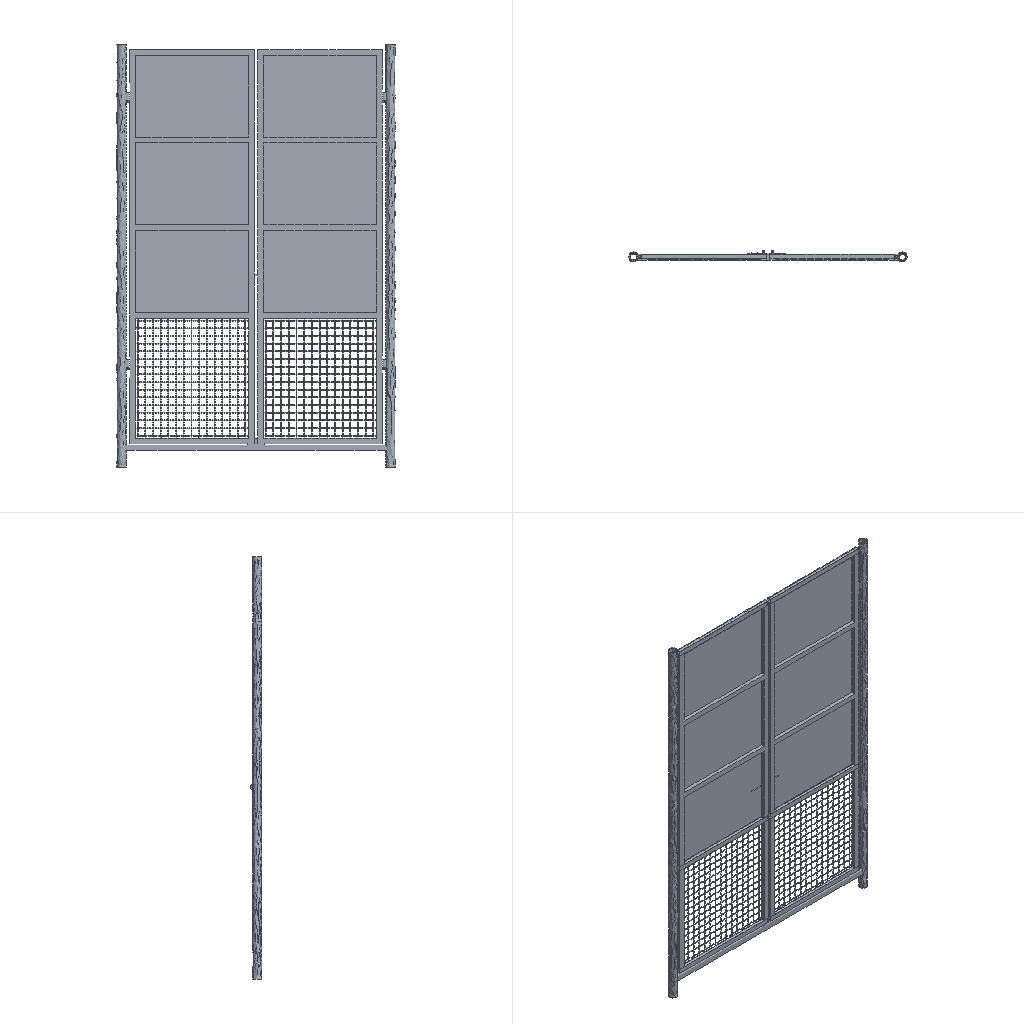Simulation study | ansys workbench
Ansys APDL input file, long lists of numbers shortened:
/batch
/config,noeldb,1     ! force off writing results to database
*get,_wallstrt,active,,time,wall
! ANSYS input file written by Workbench version 2022 R1
! File used for geometry attach:
/title,wbnew--____ (B5)
! ****** Begin Custom Load Command Snippet ******
/COM, ACT Extensions:
/COM,     LSDYNA, 2021.1
/COM,
! ****** End   Custom Load Command Snippet ******
*DIM,_wb_ProjectScratch_dir,string,248
_wb_ProjectScratch_dir(1) = ''
*DIM,_wb_SolverFiles_dir,string,248
_wb_SolverFiles_dir(1) = ''
*DIM,_wb_userfiles_dir,string,248
_wb_userfiles_dir(1) = ''
/com,--- Data in consistent NMM units. See Solving Units in the help system for more information.
/units,MPA
/nopr
/wb,file,start              !  signify a WB generated input file
/prep7
! Turn off shape checking because checks already performed inside WB mesher.
! See help system for more information.
SHPP,OFF,,NOWARN
/nolist
etcon,set             ! allow ANSYS to choose best KEYOP's for 180x elements, resets any applicable keyopt to MAPDL defaults
/com,*********** Nodes for the whole assembly ***********
nblock,3,,124940
(1i9,3e20.9e3)
    95183     1.797300000E+03     1.700000000E+01    -2.052050000E+03
! (113581 more lines like these left out)
-1
/wb,elem,start            !  set before creation of elements
/com,*********** Elements for Body 1 "SYS|__" ***********
et,1,187
eblock,19,solid,,19204
(19i9)
        1        1        1        1        0        0        0        0       10        0        1     5714     7694     5747     7607    34581    34743    34575    34580
! (38407 more lines like these left out)
-1
/com,*********** Elements for Body 2 "SYS|__[3]" ***********
et,2,187
eblock,19,solid,,157
(19i9)
        2        2        2        2        0        0        0        0       10        0    20395    46682    46735    46707    46755    46784    46920    46783    46785
! (313 more lines like these left out)
-1
/com,*********** Elements for Body 3 "SYS|__[4]" ***********
et,3,187
eblock,19,solid,,16906
(19i9)
        3        3        3        3        0        0        0        0       10        0    20552    49346    55490    49378    49532    71070    71330    71063    71064
! (33811 more lines like these left out)
-1
/com,*********** Elements for Body 4 "SYS|__[6]" ***********
et,4,187
eblock,19,solid,,149
(19i9)
        4        4        4        4        0        0        0        0       10        0    39210    95194    95223    95249    95233    95323    95469    95326    95324
! (297 more lines like these left out)
-1
/com,*********** Elements for Body 5 "SYS|__1" ***********
et,5,187
eblock,19,solid,,6702
(19i9)
        5        5        5        5        0        0        0        0       10        0    39359    95883    97753    95886    96700    99984   100001    99980    99981
! (13403 more lines like these left out)
-1
/com,*********** Elements for Body 6 "SYS|__1[2]" ***********
et,6,187
eblock,19,solid,,6145
(19i9)
        6        6        6        6        0        0        0        0       10        0    46061   109296   109671   109477   109542   112695   113726   112692   112693
! (12289 more lines like these left out)
-1
/wb,elem,end               !  done creating elements
/com,*********** Send User Defined Coordinate System(s) ***********
csys,0
toffst,273.15,  ! Temperature offset from absolute zero
/com,*********** Set Reference Temperature ***********
tref,22.
/wb,mat,start              !  starting to send materials
/com,*********** Send Materials ***********
Temperature = 'TEMP' ! Temperature
MP,DENS,1,7.85e-09,	! tonne mm^-3
MP,ALPX,1,1.2e-05,	! C^-1
MP,C,1,434000000,	! mm^2 s^-2 C^-1
MP,KXX,1,60.5,	! tonne mm s^-3 C^-1
MP,RSVX,1,0.00017,	! ohm mm
MP,EX,1,200000,	! tonne s^-2 mm^-1
MP,NUXY,1,0.3,
MP,MURX,1,10000,
Temperature = 'TEMP' ! Temperature
MP,DENS,2,7.85e-09,	! tonne mm^-3
MP,ALPX,2,1.2e-05,	! C^-1
MP,C,2,434000000,	! mm^2 s^-2 C^-1
MP,KXX,2,60.5,	! tonne mm s^-3 C^-1
MP,RSVX,2,0.00017,	! ohm mm
MP,EX,2,200000,	! tonne s^-2 mm^-1
MP,NUXY,2,0.3,
MP,MURX,2,10000,
Temperature = 'TEMP' ! Temperature
MP,DENS,3,7.85e-09,	! tonne mm^-3
MP,ALPX,3,1.2e-05,	! C^-1
MP,C,3,434000000,	! mm^2 s^-2 C^-1
MP,KXX,3,60.5,	! tonne mm s^-3 C^-1
MP,RSVX,3,0.00017,	! ohm mm
MP,EX,3,200000,	! tonne s^-2 mm^-1
MP,NUXY,3,0.3,
MP,MURX,3,10000,
Temperature = 'TEMP' ! Temperature
MP,DENS,4,7.85e-09,	! tonne mm^-3
MP,ALPX,4,1.2e-05,	! C^-1
MP,C,4,434000000,	! mm^2 s^-2 C^-1
MP,KXX,4,60.5,	! tonne mm s^-3 C^-1
MP,RSVX,4,0.00017,	! ohm mm
MP,EX,4,200000,	! tonne s^-2 mm^-1
MP,NUXY,4,0.3,
MP,MURX,4,10000,
Temperature = 'TEMP' ! Temperature
MP,DENS,5,7.85e-09,	! tonne mm^-3
MP,ALPX,5,1.2e-05,	! C^-1
MP,C,5,434000000,	! mm^2 s^-2 C^-1
MP,KXX,5,60.5,	! tonne mm s^-3 C^-1
MP,RSVX,5,0.00017,	! ohm mm
MP,EX,5,200000,	! tonne s^-2 mm^-1
MP,NUXY,5,0.3,
MP,MURX,5,10000,
Temperature = 'TEMP' ! Temperature
MP,DENS,6,7.85e-09,	! tonne mm^-3
MP,ALPX,6,1.2e-05,	! C^-1
MP,C,6,434000000,	! mm^2 s^-2 C^-1
MP,KXX,6,60.5,	! tonne mm s^-3 C^-1
MP,RSVX,6,0.00017,	! ohm mm
MP,EX,6,200000,	! tonne s^-2 mm^-1
MP,NUXY,6,0.3,
MP,MURX,6,10000,
/wb,mat,end                !  done sending materials
!************************* Model Summary ********************
!SYS|__,	结构钢,	matid,	1
!SYS|__[3],	结构钢,	matid,	2
!SYS|__[4],	结构钢,	matid,	3
!SYS|__[6],	结构钢,	matid,	4
!SYS|__1,	结构钢,	matid,	5
!SYS|__1[2],	结构钢,	matid,	6
!************************* End Model Summary ********************
! get the diagonal of the bounding box. Needed later for other things
*get,_xmin,node,,mnloc,x
*get,_ymin,node,,mnloc,y
*get,_zmin,node,,mnloc,z
*get,_xmax,node,,mxloc,x
*get,_ymax,node,,mxloc,y
*get,_zmax,node,,mxloc,z
_ASMDIAG=(_xmax-_xmin)*(_xmax-_xmin)+(_ymax-_ymin)*(_ymax-_ymin)+(_zmax-_zmin)*(_zmax-_zmin)
_ASMDIAG=SQRT(_ASMDIAG)
/wb,contact,start          !  starting to send contact
/com,*********** Create Contact "接触区域 7" ***********
/com,            Real Constant Set For Above Contact Is 8 & 7
*set,tid,8
*set,cid,7
r,tid
r,cid
et,tid,170
et,cid,174
eblock,10,,,82
(15i9)
    98788        8        8        8        0     4815     4811     5592     5592    30429    30434     5592    30468
! (81 more lines like these left out)
-1
eblock,10,,,82
(15i9)
    98870        7        7        7        0     4815     4811     5592     5592    30429    30434     5592    30468
! (81 more lines like these left out)
-1
eblock,10,,,77
(15i9)
    98952        7        8        7        0    46680    46679    46708    46708    46767    46771    46708    46775
! (76 more lines like these left out)
-1
eblock,10,,,77
(15i9)
    99029        8        7        8        0    46680    46679    46708    46708    46767    46771    46708    46775
! (76 more lines like these left out)
-1
keyo,cid,8,2               ! auto create asymmetric contact (from Program Controlled setting)
keyo,cid,10,0              ! adjust contact stiffness each NR iteration (from Program Controlled setting)
keyo,cid,12,5              ! bonded always
keyo,cid,18,1              ! small sliding turned on by application
keyo,cid,2,0               ! augmented Lagrange (from Program Controlled setting)
keyo,cid,4,0               ! on Gauss point (from Program Controlled setting)
keyo,cid,9,1               ! ignore initial gaps/penetration
keyo,cid,7,0               ! No Prediction
rmod,tid,3,10.      ! FKN
rmod,tid,5,0.       ! ICONT
rmod,tid,6,0.       ! PINB
rmod,tid,10,0.      ! CNOF
rmod,tid,12,0.      ! FKT
rmod,tid,36,85      ! WB DSID
rmod,cid,3,10.      ! FKN
rmod,cid,5,0.       ! ICONT
rmod,cid,6,0.       ! PINB
rmod,cid,10,0.      ! CNOF
rmod,cid,12,0.      ! FKT
rmod,cid,36,85      ! WB DSID
/com,*********** Create Contact "接触区域 8" ***********
/com,            Real Constant Set For Above Contact Is 10 & 9
*set,tid,10
*set,cid,9
r,tid
r,cid
et,tid,170
et,cid,174
eblock,10,,,174
(15i9)
    99106       10       10       10        0     4534     4556     4535     4535    29359    29373     4535    29358
! (173 more lines like these left out)
-1
eblock,10,,,174
(15i9)
    99280        9        9        9        0     4534     4556     4535     4535    29359    29373     4535    29358
! (173 more lines like these left out)
-1
eblock,10,,,21
(15i9)
    99454        9       10        9        0    95188    95189    95190    95190    95291    95298    95190    95292
! (20 more lines like these left out)
-1
eblock,10,,,21
(15i9)
    99475       10        9       10        0    95188    95189    95190    95190    95291    95298    95190    95292
! (20 more lines like these left out)
-1
keyo,cid,8,2               ! auto create asymmetric contact (from Program Controlled setting)
keyo,cid,10,0              ! adjust contact stiffness each NR iteration (from Program Controlled setting)
keyo,cid,12,5              ! bonded always
keyo,cid,18,1              ! small sliding turned on by application
keyo,cid,2,0               ! augmented Lagrange (from Program Controlled setting)
keyo,cid,4,0               ! on Gauss point (from Program Controlled setting)
keyo,cid,9,1               ! ignore initial gaps/penetration
keyo,cid,7,0               ! No Prediction
rmod,tid,3,10.      ! FKN
rmod,tid,5,0.       ! ICONT
rmod,tid,6,0.       ! PINB
rmod,tid,10,0.      ! CNOF
rmod,tid,12,0.      ! FKT
rmod,tid,36,88      ! WB DSID
rmod,cid,3,10.      ! FKN
rmod,cid,5,0.       ! ICONT
rmod,cid,6,0.       ! PINB
rmod,cid,10,0.      ! CNOF
rmod,cid,12,0.      ! FKT
rmod,cid,36,88      ! WB DSID
/com,*********** Create Contact "接触区域 9" ***********
/com,            Real Constant Set For Above Contact Is 12 & 11
*set,tid,12
*set,cid,11
r,tid
r,cid
et,tid,170
et,cid,174
eblock,10,,,145
(15i9)
    99496       12       12       12        0     6756        9     6755     6755     7897     7896     6755    40777
! (144 more lines like these left out)
-1
eblock,10,,,145
(15i9)
    99641       11       11       11        0     6756        9     6755     6755     7897     7896     6755    40777
! (144 more lines like these left out)
-1
eblock,10,,,253
(15i9)
    99786       11       12       11        0   109149   109152   110259   110259   111453   111472   110259   111456
! (252 more lines like these left out)
-1
eblock,10,,,253
(15i9)
   100039       12       11       12        0   109149   109152   110259   110259   111453   111472   110259   111456
! (252 more lines like these left out)
-1
keyo,cid,8,2               ! auto create asymmetric contact (from Program Controlled setting)
keyo,cid,10,0              ! adjust contact stiffness each NR iteration (from Program Controlled setting)
keyo,cid,12,5              ! bonded always
keyo,cid,18,1              ! small sliding turned on by application
keyo,cid,2,0               ! augmented Lagrange (from Program Controlled setting)
keyo,cid,4,0               ! on Gauss point (from Program Controlled setting)
keyo,cid,9,1               ! ignore initial gaps/penetration
keyo,cid,7,0               ! No Prediction
rmod,tid,3,10.      ! FKN
rmod,tid,5,0.       ! ICONT
rmod,tid,6,0.       ! PINB
rmod,tid,10,0.      ! CNOF
rmod,tid,12,0.      ! FKT
rmod,tid,36,91      ! WB DSID
rmod,cid,3,10.      ! FKN
rmod,cid,5,0.       ! ICONT
rmod,cid,6,0.       ! PINB
rmod,cid,10,0.      ! CNOF
rmod,cid,12,0.      ! FKT
rmod,cid,36,91      ! WB DSID
/com,*********** Create Contact "接触区域 14" ***********
/com,            Real Constant Set For Above Contact Is 14 & 13
*set,tid,14
*set,cid,13
r,tid
r,cid
et,tid,170
et,cid,174
eblock,10,,,85
(15i9)
   100292       14       14       14        0    46737    46714    46753    46753    46953    46955    46753    47036
! (84 more lines like these left out)
-1
eblock,10,,,85
(15i9)
   100377       13       13       13        0    46737    46714    46753    46753    46953    46955    46753    47036
! (84 more lines like these left out)
-1
eblock,10,,,144
(15i9)
   100462       13       14       13        0    47082    47078    47072    47072    55787    55744    47072    55746
! (143 more lines like these left out)
-1
eblock,10,,,144
(15i9)
   100606       14       13       14        0    47082    47078    47072    47072    55787    55744    47072    55746
! (143 more lines like these left out)
-1
keyo,cid,8,2               ! auto create asymmetric contact (from Program Controlled setting)
keyo,cid,10,0              ! adjust contact stiffness each NR iteration (from Program Controlled setting)
keyo,cid,12,5              ! bonded always
keyo,cid,18,1              ! small sliding turned on by application
keyo,cid,2,0               ! augmented Lagrange (from Program Controlled setting)
keyo,cid,4,0               ! on Gauss point (from Program Controlled setting)
keyo,cid,9,1               ! ignore initial gaps/penetration
keyo,cid,7,0               ! No Prediction
rmod,tid,3,10.      ! FKN
rmod,tid,5,0.       ! ICONT
rmod,tid,6,0.       ! PINB
rmod,tid,10,0.      ! CNOF
rmod,tid,12,0.      ! FKT
rmod,tid,36,106     ! WB DSID
rmod,cid,3,10.      ! FKN
rmod,cid,5,0.       ! ICONT
rmod,cid,6,0.       ! PINB
rmod,cid,10,0.      ! CNOF
rmod,cid,12,0.      ! FKT
rmod,cid,36,106     ! WB DSID
/com,*********** Create Contact "接触区域 21" ***********
/com,            Real Constant Set For Above Contact Is 16 & 15
*set,tid,16
*set,cid,15
r,tid
r,cid
et,tid,170
et,cid,174
eblock,10,,,130
(15i9)
   100750       16       16       16        0    49254    49260    55435    55435    70455    70529    55435    70461
! (129 more lines like these left out)
-1
eblock,10,,,130
(15i9)
   100880       15       15       15        0    49254    49260    55435    55435    70455    70529    55435    70461
! (129 more lines like these left out)
-1
eblock,10,,,21
(15i9)
   101010       15       16       15        0    95188    95189    95190    95190    95291    95298    95190    95292
! (20 more lines like these left out)
-1
eblock,10,,,21
(15i9)
   101031       16       15       16        0    95188    95189    95190    95190    95291    95298    95190    95292
! (20 more lines like these left out)
-1
keyo,cid,8,2               ! auto create asymmetric contact (from Program Controlled setting)
keyo,cid,10,0              ! adjust contact stiffness each NR iteration (from Program Controlled setting)
keyo,cid,12,5              ! bonded always
keyo,cid,18,1              ! small sliding turned on by application
keyo,cid,2,0               ! augmented Lagrange (from Program Controlled setting)
keyo,cid,4,0               ! on Gauss point (from Program Controlled setting)
keyo,cid,9,1               ! ignore initial gaps/penetration
keyo,cid,7,0               ! No Prediction
rmod,tid,3,10.      ! FKN
rmod,tid,5,0.       ! ICONT
rmod,tid,6,0.       ! PINB
rmod,tid,10,0.      ! CNOF
rmod,tid,12,0.      ! FKT
rmod,tid,36,127     ! WB DSID
rmod,cid,3,10.      ! FKN
rmod,cid,5,0.       ! ICONT
rmod,cid,6,0.       ! PINB
rmod,cid,10,0.      ! CNOF
rmod,cid,12,0.      ! FKT
rmod,cid,36,127     ! WB DSID
/com,*********** Create Contact "接触区域 22" ***********
/com,            Real Constant Set For Above Contact Is 18 & 17
*set,tid,18
*set,cid,17
r,tid
r,cid
et,tid,170
et,cid,174
eblock,10,,,147
(15i9)
   101052       18       18       18        0    49358    55448    49366    49366    71173    71233    49366    71168
! (146 more lines like these left out)
-1
eblock,10,,,147
(15i9)
   101199       17       17       17        0    49358    55448    49366    49366    71173    71233    49366    71168
! (146 more lines like these left out)
-1
eblock,10,,,269
(15i9)
   101346       17       18       17        0    95613    95614    95883    95883    98010    98015    95883    98012
! (268 more lines like these left out)
-1
eblock,10,,,269
(15i9)
   101615       18       17       18        0    95613    95614    95883    95883    98010    98015    95883    98012
! (268 more lines like these left out)
-1
keyo,cid,8,2               ! auto create asymmetric contact (from Program Controlled setting)
keyo,cid,10,0              ! adjust contact stiffness each NR iteration (from Program Controlled setting)
keyo,cid,12,5              ! bonded always
keyo,cid,18,1              ! small sliding turned on by application
keyo,cid,2,0               ! augmented Lagrange (from Program Controlled setting)
keyo,cid,4,0               ! on Gauss point (from Program Controlled setting)
keyo,cid,9,1               ! ignore initial gaps/penetration
keyo,cid,7,0               ! No Prediction
rmod,tid,3,10.      ! FKN
rmod,tid,5,0.       ! ICONT
rmod,tid,6,0.       ! PINB
rmod,tid,10,0.      ! CNOF
rmod,tid,12,0.      ! FKT
rmod,tid,36,130     ! WB DSID
rmod,cid,3,10.      ! FKN
rmod,cid,5,0.       ! ICONT
rmod,cid,6,0.       ! PINB
rmod,cid,10,0.      ! CNOF
rmod,cid,12,0.      ! FKT
rmod,cid,36,130     ! WB DSID
/com,*********** Create Contact "接触区域 27" ***********
/com,            Real Constant Set For Above Contact Is 20 & 19
*set,tid,20
*set,cid,19
r,tid
r,cid
et,tid,170
et,cid,174
eblock,10,,,4
(15i9)
   101884       20       20       20        0    95240    95242    95258    95258    95530    95538    95258    95531
   101885       20       20       20        0    95227    95242    95240    95240    95488    95530    95240    95487
   101886       20       20       20        0    95193    95240    95200    95200    95316    95360    95200    95315
   101887       20       20       20        0    95200    95240    95258    95258    95360    95531    95258    95361
-1
eblock,10,,,4
(15i9)
   101888       19       19       19        0    95240    95242    95258    95258    95530    95538    95258    95531
   101889       19       19       19        0    95227    95242    95240    95240    95488    95530    95240    95487
   101890       19       19       19        0    95193    95240    95200    95200    95316    95360    95200    95315
   101891       19       19       19        0    95200    95240    95258    95258    95360    95531    95258    95361
-1
eblock,10,,,38
(15i9)
   101892       19       20       19        0    95795    96189    96188    96188    99200   101510    96188    99199
! (37 more lines like these left out)
-1
eblock,10,,,38
(15i9)
   101930       20       19       20        0    95795    96189    96188    96188    99200   101510    96188    99199
! (37 more lines like these left out)
-1
keyo,cid,8,2               ! auto create asymmetric contact (from Program Controlled setting)
keyo,cid,10,0              ! adjust contact stiffness each NR iteration (from Program Controlled setting)
keyo,cid,12,5              ! bonded always
keyo,cid,18,1              ! small sliding turned on by application
keyo,cid,2,0               ! augmented Lagrange (from Program Controlled setting)
keyo,cid,4,0               ! on Gauss point (from Program Controlled setting)
keyo,cid,9,1               ! ignore initial gaps/penetration
keyo,cid,7,0               ! No Prediction
rmod,tid,3,10.      ! FKN
rmod,tid,5,0.       ! ICONT
rmod,tid,6,0.       ! PINB
rmod,tid,10,0.      ! CNOF
rmod,tid,12,0.      ! FKT
rmod,tid,36,145     ! WB DSID
rmod,cid,3,10.      ! FKN
rmod,cid,5,0.       ! ICONT
rmod,cid,6,0.       ! PINB
rmod,cid,10,0.      ! CNOF
rmod,cid,12,0.      ! FKT
rmod,cid,36,145     ! WB DSID
/com,*********** Create Contact "接触区域 28" ***********
/com,            Real Constant Set For Above Contact Is 22 & 21
*set,tid,22
*set,cid,21
r,tid
r,cid
et,tid,170
et,cid,174
eblock,10,,,4
(15i9)
   101968       22       22       22        0    95226    95225    95241    95241    95478    95479    95241    95485
   101969       22       22       22        0    95241    95225    95257    95257    95479    95480    95257    95535
   101970       22       22       22        0    95225    95201    95257    95257    95365    95366    95257    95480
   101971       22       22       22        0    95216    95201    95225    95225    95364    95365    95225    95434
-1
eblock,10,,,4
(15i9)
   101972       21       21       21        0    95226    95225    95241    95241    95478    95479    95241    95485
   101973       21       21       21        0    95241    95225    95257    95257    95479    95480    95257    95535
   101974       21       21       21        0    95225    95201    95257    95257    95365    95366    95257    95480
   101975       21       21       21        0    95216    95201    95225    95225    95364    95365    95225    95434
-1
eblock,10,,,25
(15i9)
   101976       21       22       21        0   109377   109729   109728   109728   113201   114867   109728   113200
! (24 more lines like these left out)
-1
eblock,10,,,25
(15i9)
   102001       22       21       22        0   109377   109729   109728   109728   113201   114867   109728   113200
! (24 more lines like these left out)
-1
keyo,cid,8,2               ! auto create asymmetric contact (from Program Controlled setting)
keyo,cid,10,0              ! adjust contact stiffness each NR iteration (from Program Controlled setting)
keyo,cid,12,5              ! bonded always
keyo,cid,18,1              ! small sliding turned on by application
keyo,cid,2,0               ! augmented Lagrange (from Program Controlled setting)
keyo,cid,4,0               ! on Gauss point (from Program Controlled setting)
keyo,cid,9,1               ! ignore initial gaps/penetration
keyo,cid,7,0               ! No Prediction
rmod,tid,3,10.      ! FKN
rmod,tid,5,0.       ! ICONT
rmod,tid,6,0.       ! PINB
rmod,tid,10,0.      ! CNOF
rmod,tid,12,0.      ! FKT
rmod,tid,36,148     ! WB DSID
rmod,cid,3,10.      ! FKN
rmod,cid,5,0.       ! ICONT
rmod,cid,6,0.       ! PINB
rmod,cid,10,0.      ! CNOF
rmod,cid,12,0.      ! FKT
rmod,cid,36,148     ! WB DSID
nsel,all
esel,all
/wb,contact,end            !  done creating contacts
/golist
/wb,load,start             !  starting to send loads
/com,*********** Fixed Supports ***********
CMBLOCK,_FIXEDSU,NODE,      414
(8i10)
     95655     95656     95657     95658     95659     95660     95661     95662
! (51 more lines like these left out)
cmsel,s,_FIXEDSU
d,all,all
nsel,all
/com,*********** Define Force Using Surface Effect Elements ***********
local,12,0,0.,0.,0.,0.,0.,0.
csys,0
et,23,154
eblock,10,,,10352
(15i9)
   102026       23       23       23       12      334      333     5555     5555    10364    10371     5555    10377
! (10351 more lines like these left out)
-1
esel,s,type,,23
keyop,23,2,1                ! Apply load in local coordinate system
keyop,23,7,1                ! Use original area so load is constant in large deformation
esel,all
/gst,on,on
fini
*get,_numnode,node,0,count
*get,_numelem,elem,0,count
*get, _MAXELEMNUM, elem, 0, NUM, MAX
*get, _MAXNODENUM, node, 0, NUM, MAX
*get, _MAXELEMTYPE, etyp, 0, NUM, MAX
*get, _MAXREALCONST, real, 0, NUM, MAX
/go
/wb,load,end               !  done creating loads
/com,--- Number of total nodes = %_numnode%
/com,--- Number of contact elements = 13590
/com,--- Number of spring elements = 0
/com,--- Number of bearing elements = 0
/com,--- Number of solid elements = 49263
/com,--- Number of condensed parts = 0
/com,--- Number of total elements = %_numelem%
*get,_wallbsol,active,,time,wall
/com,****************************************************************************
/com,*************************    SOLUTION       ********************************
/com,****************************************************************************
/solu
antype,0                   ! static analysis
_thickRatio=  0     ! Ratio of thick parts in the model
eqsl,sparse,,,,,1
cntr,print,1               ! print out contact info and also make no initial contact an error
dmpoption,emat,no             ! Don't combine emat file for DANSYS
dmpoption,esav,no             ! Don't combine esav file for DANSYS
nldiag,cont,iter           ! print out contact info each equilibrium iteration
rescontrol,,none                 ! Do not keep any restart files
/com,****************************************************
/com,******************* SOLVE FOR LS 1 OF 1 ****************
esel,s,type,,23
nsle
sfe,all,1,pres,1,0.
sfe,all,2,pres,1,-1.4797955785793e-004
sfe,all,3,pres,1,0.
nsel,all
esel,all
/nopr
/gopr
nsub,1,1,1
time,1.
outres,erase
outres,all,none
outres,nsol,all,
outres,rsol,all
outres,eangl,all
outres,etmp,all
outres,veng,all
outres,strs,all,
outres,epel,all,
outres,eppl,all,
outres,cont,all,
! *********** WB SOLVE COMMAND ***********
! check interactive state
*get,ANSINTER_,active,,int
*if,ANSINTER_,ne,0,then
/eof
*endif
solve
/com *************** Write FE CONNECTORS *********
CEWRITE,file,ce,,INTE
/com,****************************************************
/com,*************** FINISHED SOLVE FOR LS 1 *************
*get,_wallasol,active,,time,wall
/nopr
*get,_numnode,node,0,count
*get,_numelem,elem,0,count
*get, _MAXELEMNUM, elem, 0, NUM, MAX
*get, _MAXNODENUM, node, 0, NUM, MAX,,,INTERNAL
*get, _MAXELEMTYPE, etyp, 0, NUM, MAX
*get, _MAXREALCONST, real, 0, NUM, MAX
/gopr
/post1
xmlo,ENCODING,ISO-8859-1
xmlo,parm
/xml,parm,xml
fini
/gopr
*get,_walldone,active,,time,wall
_preptime=(_wallbsol-_wallstrt)*3600
_solvtime=(_wallasol-_wallbsol)*3600
_posttime=(_walldone-_wallasol)*3600
_totaltim=(_walldone-_wallstrt)*3600
*get,_dlbratio,active,0,solu,dlbr
*get,_combtime,active,0,solu,comb
*get,_ssmode,active,0,solu,ssmm
*get,_ndofs,active,0,solu,ndof
*get,_sol_end_time,active,0,set,time
*if,_sol_end_time,eq,1.,then
/fclean				!clean distributed files
*endif
/com,--- Total number of nodes = %_numnode%
/com,--- Total number of elements = %_numelem%
/com,--- Element load balance ratio = %_dlbratio%
/com,--- Time to combine distributed files = %_combtime%
/com,--- Sparse memory mode = %_ssmode%
/com,--- Number of DOF = %_ndofs%
/wb,file,end               ! done with WB generated input